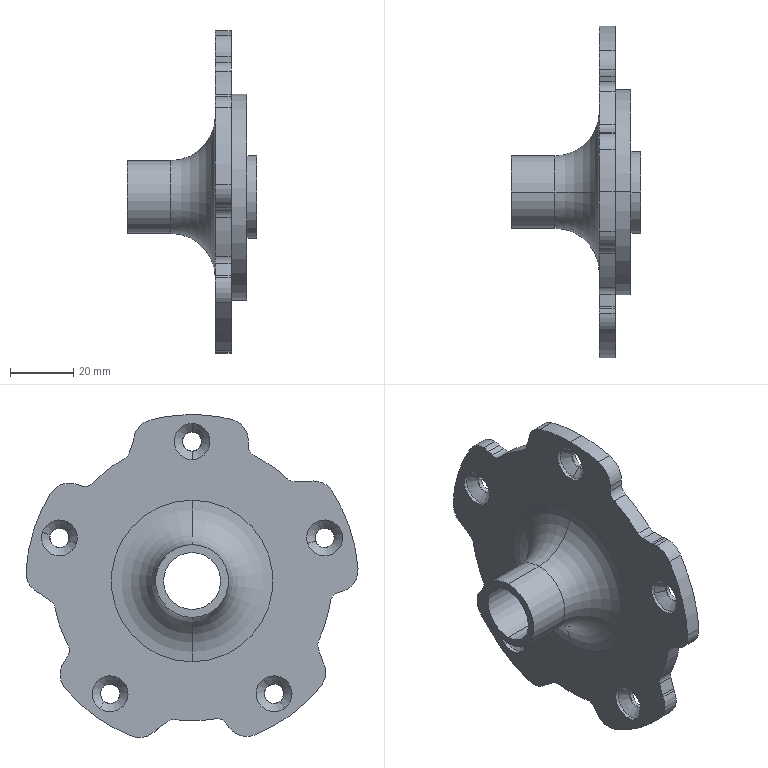Part | STEP file | Completa.sldasm-Part-2_Valor predeterminado | 1 solid | 103 faces | box 40.919 x 104.793 x 101.882 mm | volume 59946 mm3 | cylinder 66 | plane 15 | torus 12 | cone 10 | commonest cylinder face diameters 6.496 x15 14 x12 6 x10 11.34 x10 105 x6 88.221 x5